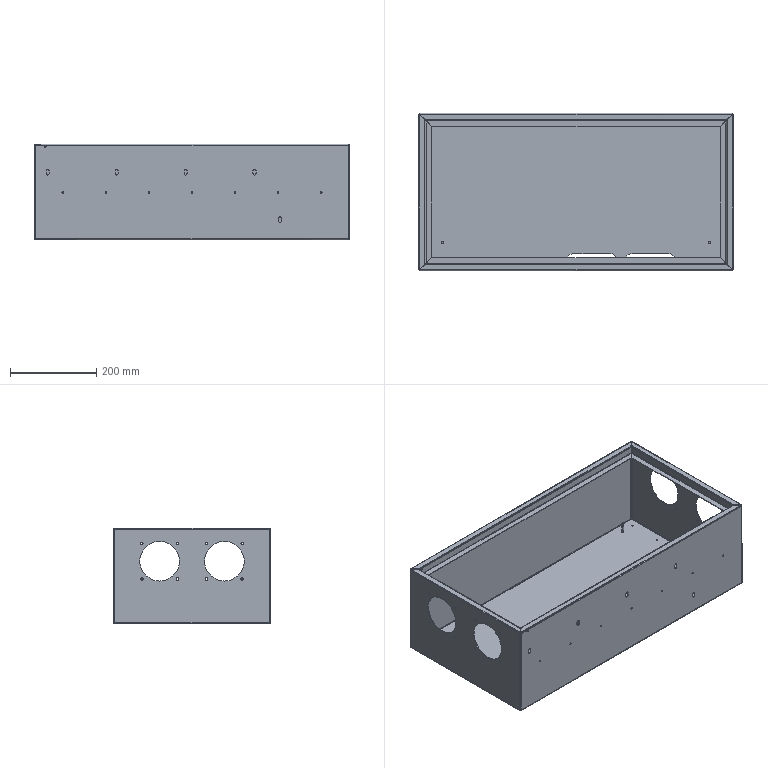Part | SolidWorks | features HoleWzd 6, ICE 4, EdgeFlange 3, FlatPattern 1, SheetMetal 1, SolidToSheetMetal 1 | 5 solids | 305 faces | box 730 x 365 x 221.5 mm | volume 1200734 mm3 | cylinder 149 | plane 124 | spline 32 | commonest cylinder face diameters 3.3 x42 5.5 x32 1.473 x16 4.473 x16 7 x15 5 x8